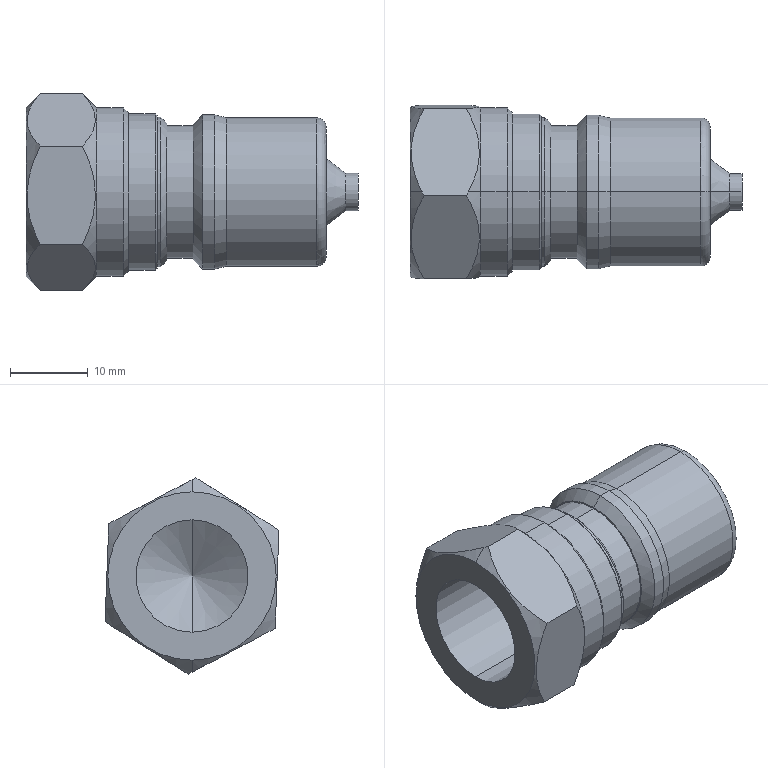Part | STEP file | 4-20.sldasm-Part-56 | 1 solid | 49 faces | box 42.596 x 22.32 x 25.204 mm | volume 9972 mm3 | cone 18 | cylinder 16 | plane 13 | torus 2 | commonest cylinder face diameters 4.775 x2 14.417 x2 17.043 x2 19.05 x2 19.152 x2 19.812 x2